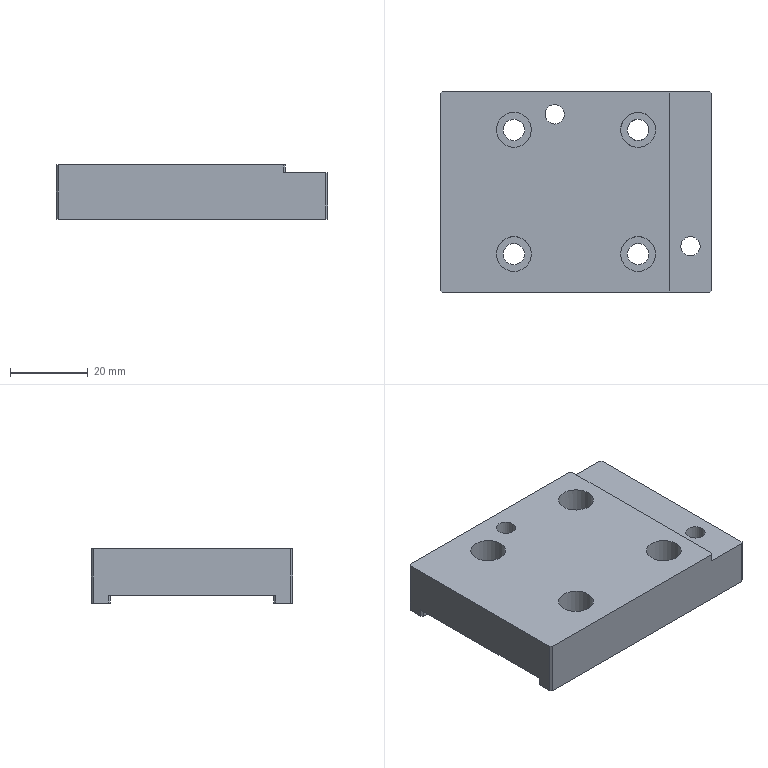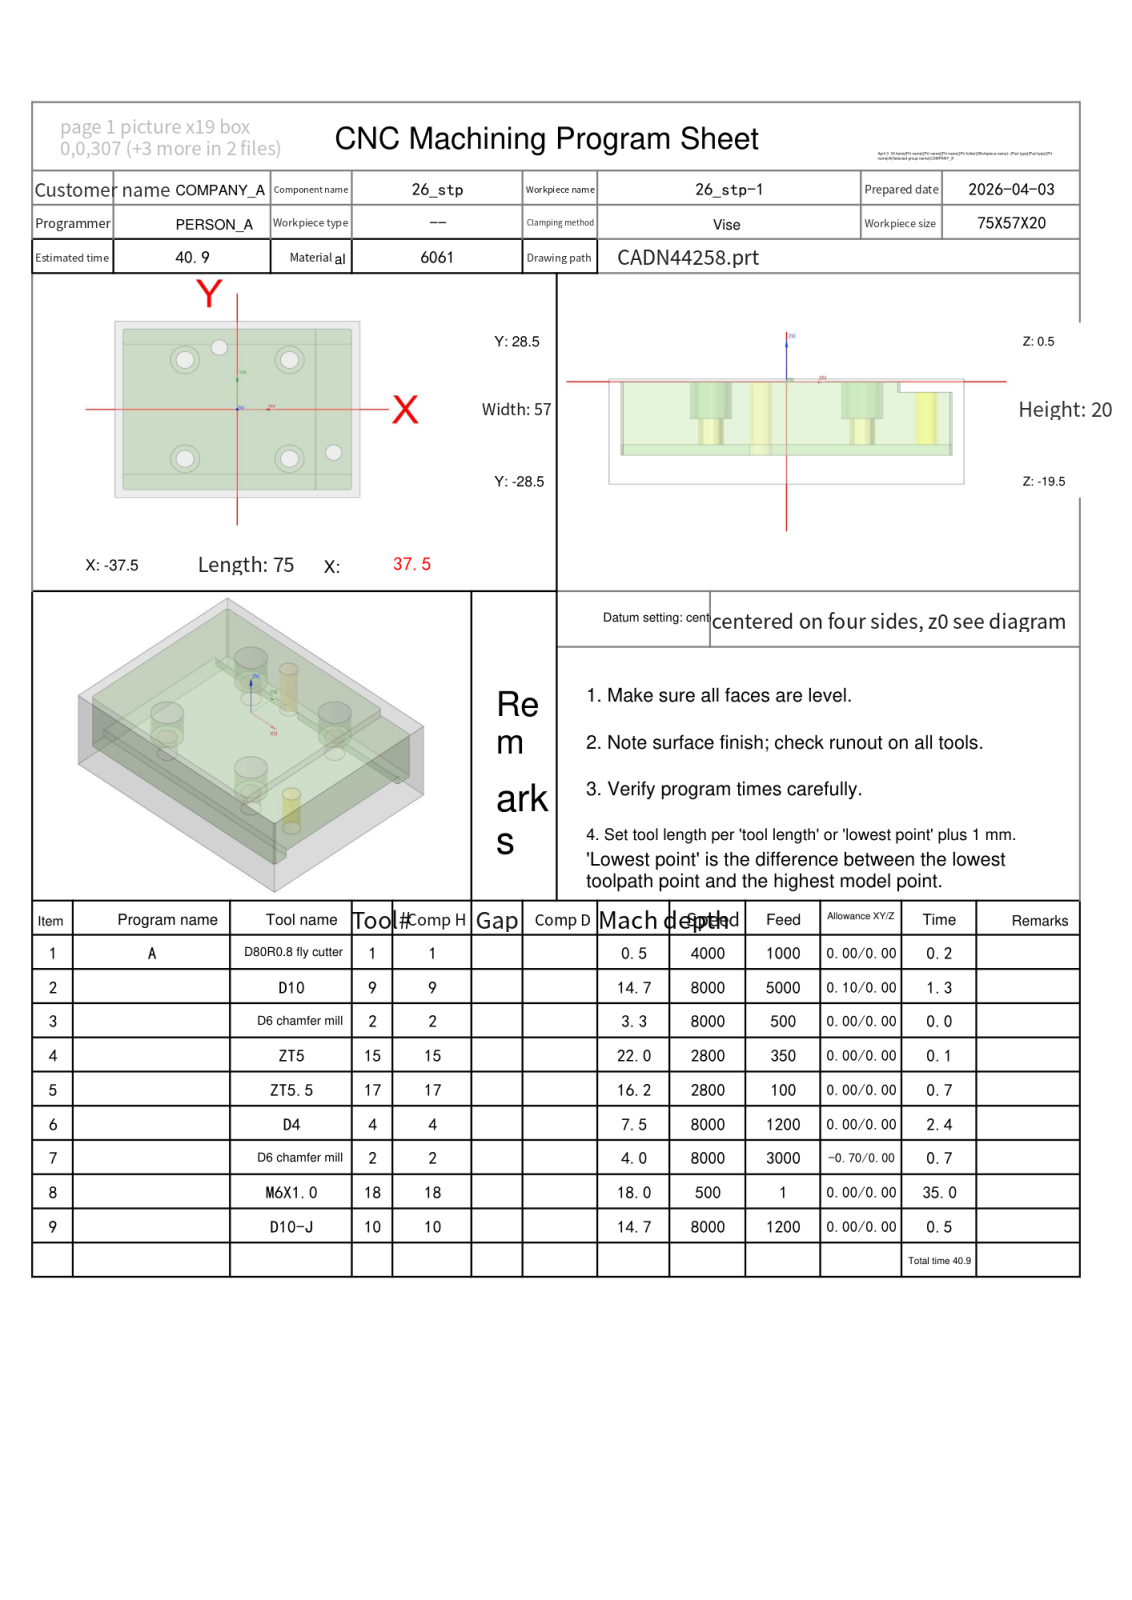NC program | NX | posted by the shop | part box 70 x 52 x 14 mm
Whole program, first 1466 of 2128 lines:
%
O0001
(Machine time: 75.66 MIN)
(===Total Tool:8===)
(T1=D80R0.8 fly cutter D=80.  R=0.8  D-  H01 Z=0.    )
(T9=D10     D=10.  R=0.   D-  H09 Z=-14.2 )
(T2=D6 chamfer mill   D=6.   R=0.   D-  H02 Z=-3.5  )
(T15=ZT5    D=5.   DR_a=118 D-  H15 Z=-21.5 )
(T17=ZT5.5  D=5.5  DR_a=118 D-  H17 Z=-15.65)
(T4=D4      D=4.   R=0.   D4  H04 Z=-7.   )
(T18=M6X1.0 D=5.   DR_a=180 D-  H18 Z=-17.5 )
(T10=D10-J  D=10.  R=0.   D10 H10 Z=-14.2 )
G80 G90 G17 G49 G40
G91 G28 Z0
M01
N1 T01 M06
(D80R0.8 fly cutter  D=80. R=0.8 H=01 ce=0.00 di=0.00)
G00 G90 G54 X-80. Y0.0 M03 S4000
G43 H01 Z20.
M08
Z2.
G01 Z0.0 F1000.
X-75.
X75.
X80.
Z2.
G00 Z20.
G91 G28 Z0.0
M05
M09
G91 G28 Z0.0
M01
N2 T09 M06
(D10  D=10. R=0. H=09 ce=0.10 di=0.00)
G00 G90 G54 X0.0 Y31.1 M03 S8000
G43 H09 Z20.
M08
Z.5
G01 X34.5 Z.403 F5000.
G02 X38.106 Y29.606 Z.392 I0.0 J-5.1
G01 X38.606 Y29.106 Z.39
G02 X40.1 Y25.5 Z.378 I-3.606 J-3.606
G01 Y-25.5 Z.235
G02 X38.606 Y-29.106 Z.224 I-5.1 J0.0
G01 X38.106 Y-29.606 Z.222
G02 X34.5 Y-31.1 Z.21 I-3.606 J3.606
G01 X-34.5 Z.016
G02 X-38.106 Y-29.606 Z.005 I0.0 J5.1
G01 X-38.606 Y-29.106 Z.003
G02 X-40.1 Y-25.5 Z-.008 I3.606 J3.606
G01 Y25.5 Z-.152
G02 X-38.606 Y29.106 Z-.163 I5.1 J0.0
G01 X-38.106 Y29.606 Z-.165
G02 X-34.5 Y31.1 Z-.177 I3.606 J-3.606
G01 X34.5 Z-.371
G02 X38.106 Y29.606 Z-.382 I0.0 J-5.1
G01 X38.606 Y29.106 Z-.384
G02 X40.1 Y25.5 Z-.395 I-3.606 J-3.606
G01 Y-25.5 Z-.539
G02 X38.606 Y-29.106 Z-.55 I-5.1 J0.0
G01 X38.106 Y-29.606 Z-.552
G02 X34.5 Y-31.1 Z-.563 I-3.606 J3.606
G01 X-34.5 Z-.758
G02 X-38.106 Y-29.606 Z-.769 I0.0 J5.1
G01 X-38.606 Y-29.106 Z-.771
G02 X-40.1 Y-25.5 Z-.782 I3.606 J3.606
G01 Y25.5 Z-.926
G02 X-38.606 Y29.106 Z-.937 I5.1 J0.0
G01 X-38.106 Y29.606 Z-.939
G02 X-34.5 Y31.1 Z-.95 I3.606 J-3.606
G01 X34.5 Z-1.144
G02 X38.106 Y29.606 Z-1.156 I0.0 J-5.1
G01 X38.606 Y29.106 Z-1.158
G02 X40.1 Y25.5 Z-1.169 I-3.606 J-3.606
G01 Y-25.5 Z-1.313
G02 X38.606 Y-29.106 Z-1.324 I-5.1 J0.0
G01 X38.106 Y-29.606 Z-1.326
G02 X34.5 Y-31.1 Z-1.337 I-3.606 J3.606
G01 X-34.5 Z-1.531
G02 X-38.106 Y-29.606 Z-1.543 I0.0 J5.1
G01 X-38.606 Y-29.106 Z-1.545
G02 X-40.1 Y-25.5 Z-1.556 I3.606 J3.606
G01 Y25.5 Z-1.699
G02 X-38.606 Y29.106 Z-1.711 I5.1 J0.0
G01 X-38.106 Y29.606 Z-1.713
G02 X-34.5 Y31.1 Z-1.724 I3.606 J-3.606
G01 X34.5 Z-1.918
G02 X38.106 Y29.606 Z-1.929 I0.0 J-5.1
G01 X38.606 Y29.106 Z-1.931
G02 X40.1 Y25.5 Z-1.943 I-3.606 J-3.606
G01 Y-25.5 Z-2.086
G02 X38.606 Y-29.106 Z-2.098 I-5.1 J0.0
G01 X38.106 Y-29.606 Z-2.1
G02 X34.5 Y-31.1 Z-2.111 I-3.606 J3.606
G01 X-34.5 Z-2.305
G02 X-38.106 Y-29.606 Z-2.316 I0.0 J5.1
G01 X-38.606 Y-29.106 Z-2.318
G02 X-40.1 Y-25.5 Z-2.33 I3.606 J3.606
G01 Y25.5 Z-2.473
G02 X-38.606 Y29.106 Z-2.484 I5.1 J0.0
G01 X-38.106 Y29.606 Z-2.486
G02 X-34.5 Y31.1 Z-2.498 I3.606 J-3.606
G01 X34.5 Z-2.692
G02 X38.106 Y29.606 Z-2.703 I0.0 J-5.1
G01 X38.606 Y29.106 Z-2.705
G02 X40.1 Y25.5 Z-2.716 I-3.606 J-3.606
G01 Y-25.5 Z-2.86
G02 X38.606 Y-29.106 Z-2.871 I-5.1 J0.0
G01 X38.106 Y-29.606 Z-2.873
G02 X34.5 Y-31.1 Z-2.884 I-3.606 J3.606
G01 X-34.5 Z-3.079
G02 X-38.106 Y-29.606 Z-3.09 I0.0 J5.1
G01 X-38.606 Y-29.106 Z-3.092
G02 X-40.1 Y-25.5 Z-3.103 I3.606 J3.606
G01 Y25.5 Z-3.247
G02 X-38.606 Y29.106 Z-3.258 I5.1 J0.0
G01 X-38.106 Y29.606 Z-3.26
G02 X-34.5 Y31.1 Z-3.271 I3.606 J-3.606
G01 X34.5 Z-3.466
G02 X38.106 Y29.606 Z-3.477 I0.0 J-5.1
G01 X38.606 Y29.106 Z-3.479
G02 X40.1 Y25.5 Z-3.49 I-3.606 J-3.606
G01 Y-25.5 Z-3.634
G02 X38.606 Y-29.106 Z-3.645 I-5.1 J0.0
G01 X38.106 Y-29.606 Z-3.647
G02 X34.5 Y-31.1 Z-3.658 I-3.606 J3.606
G01 X-34.5 Z-3.852
G02 X-38.106 Y-29.606 Z-3.864 I0.0 J5.1
G01 X-38.606 Y-29.106 Z-3.866
G02 X-40.1 Y-25.5 Z-3.877 I3.606 J3.606
G01 Y25.5 Z-4.02
G02 X-38.606 Y29.106 Z-4.032 I5.1 J0.0
G01 X-38.106 Y29.606 Z-4.034
G02 X-34.5 Y31.1 Z-4.045 I3.606 J-3.606
G01 X34.5 Z-4.239
G02 X38.106 Y29.606 Z-4.25 I0.0 J-5.1
G01 X38.606 Y29.106 Z-4.252
G02 X40.1 Y25.5 Z-4.264 I-3.606 J-3.606
G01 Y-25.5 Z-4.407
G02 X38.606 Y-29.106 Z-4.419 I-5.1 J0.0
G01 X38.106 Y-29.606 Z-4.421
G02 X34.5 Y-31.1 Z-4.432 I-3.606 J3.606
G01 X-34.5 Z-4.626
G02 X-38.106 Y-29.606 Z-4.637 I0.0 J5.1
G01 X-38.606 Y-29.106 Z-4.639
G02 X-40.1 Y-25.5 Z-4.651 I3.606 J3.606
G01 Y25.5 Z-4.794
G02 X-38.606 Y29.106 Z-4.805 I5.1 J0.0
G01 X-38.106 Y29.606 Z-4.807
G02 X-34.5 Y31.1 Z-4.819 I3.606 J-3.606
G01 X34.5 Z-5.013
G02 X38.106 Y29.606 Z-5.024 I0.0 J-5.1
G01 X38.606 Y29.106 Z-5.026
G02 X40.1 Y25.5 Z-5.037 I-3.606 J-3.606
G01 Y-25.5 Z-5.181
G02 X38.606 Y-29.106 Z-5.192 I-5.1 J0.0
G01 X38.106 Y-29.606 Z-5.194
G02 X34.5 Y-31.1 Z-5.206 I-3.606 J3.606
G01 X-34.5 Z-5.4
G02 X-38.106 Y-29.606 Z-5.411 I0.0 J5.1
G01 X-38.606 Y-29.106 Z-5.413
G02 X-40.1 Y-25.5 Z-5.424 I3.606 J3.606
G01 Y25.5 Z-5.568
G02 X-38.606 Y29.106 Z-5.579 I5.1 J0.0
G01 X-38.106 Y29.606 Z-5.581
G02 X-34.5 Y31.1 Z-5.592 I3.606 J-3.606
G01 X34.5 Z-5.787
G02 X38.106 Y29.606 Z-5.798 I0.0 J-5.1
G01 X38.606 Y29.106 Z-5.8
G02 X40.1 Y25.5 Z-5.811 I-3.606 J-3.606
G01 Y-25.5 Z-5.955
G02 X38.606 Y-29.106 Z-5.966 I-5.1 J0.0
G01 X38.106 Y-29.606 Z-5.968
G02 X34.5 Y-31.1 Z-5.979 I-3.606 J3.606
G01 X-34.5 Z-6.173
G02 X-38.106 Y-29.606 Z-6.185 I0.0 J5.1
G01 X-38.606 Y-29.106 Z-6.187
G02 X-40.1 Y-25.5 Z-6.198 I3.606 J3.606
G01 Y25.5 Z-6.342
G02 X-38.606 Y29.106 Z-6.353 I5.1 J0.0
G01 X-38.106 Y29.606 Z-6.355
G02 X-34.5 Y31.1 Z-6.366 I3.606 J-3.606
G01 X34.5 Z-6.56
G02 X38.106 Y29.606 Z-6.572 I0.0 J-5.1
G01 X38.606 Y29.106 Z-6.574
G02 X40.1 Y25.5 Z-6.585 I-3.606 J-3.606
G01 Y-25.5 Z-6.728
G02 X38.606 Y-29.106 Z-6.74 I-5.1 J0.0
G01 X38.106 Y-29.606 Z-6.742
G02 X34.5 Y-31.1 Z-6.753 I-3.606 J3.606
G01 X-34.5 Z-6.947
G02 X-38.106 Y-29.606 Z-6.958 I0.0 J5.1
G01 X-38.606 Y-29.106 Z-6.96
G02 X-40.1 Y-25.5 Z-6.972 I3.606 J3.606
G01 Y25.5 Z-7.115
G02 X-38.606 Y29.106 Z-7.126 I5.1 J0.0
G01 X-38.106 Y29.606 Z-7.128
G02 X-34.5 Y31.1 Z-7.14 I3.606 J-3.606
G01 X34.5 Z-7.334
G02 X38.106 Y29.606 Z-7.345 I0.0 J-5.1
G01 X38.606 Y29.106 Z-7.347
G02 X40.1 Y25.5 Z-7.358 I-3.606 J-3.606
G01 Y-25.5 Z-7.502
G02 X38.606 Y-29.106 Z-7.513 I-5.1 J0.0
G01 X38.106 Y-29.606 Z-7.515
G02 X34.5 Y-31.1 Z-7.527 I-3.606 J3.606
G01 X-34.5 Z-7.721
G02 X-38.106 Y-29.606 Z-7.732 I0.0 J5.1
G01 X-38.606 Y-29.106 Z-7.734
G02 X-40.1 Y-25.5 Z-7.745 I3.606 J3.606
G01 Y25.5 Z-7.889
G02 X-38.606 Y29.106 Z-7.9 I5.1 J0.0
G01 X-38.106 Y29.606 Z-7.902
G02 X-34.5 Y31.1 Z-7.913 I3.606 J-3.606
G01 X34.5 Z-8.108
G02 X38.106 Y29.606 Z-8.119 I0.0 J-5.1
G01 X38.606 Y29.106 Z-8.121
G02 X40.1 Y25.5 Z-8.132 I-3.606 J-3.606
G01 Y-25.5 Z-8.276
G02 X38.606 Y-29.106 Z-8.287 I-5.1 J0.0
G01 X38.106 Y-29.606 Z-8.289
G02 X34.5 Y-31.1 Z-8.3 I-3.606 J3.606
G01 X-34.5 Z-8.494
G02 X-38.106 Y-29.606 Z-8.506 I0.0 J5.1
G01 X-38.606 Y-29.106 Z-8.508
G02 X-40.1 Y-25.5 Z-8.519 I3.606 J3.606
G01 Y25.5 Z-8.663
G02 X-38.606 Y29.106 Z-8.674 I5.1 J0.0
G01 X-38.106 Y29.606 Z-8.676
G02 X-34.5 Y31.1 Z-8.687 I3.606 J-3.606
G01 X34.5 Z-8.881
G02 X38.106 Y29.606 Z-8.893 I0.0 J-5.1
G01 X38.606 Y29.106 Z-8.895
G02 X40.1 Y25.5 Z-8.906 I-3.606 J-3.606
G01 Y-25.5 Z-9.049
G02 X38.606 Y-29.106 Z-9.061 I-5.1 J0.0
G01 X38.106 Y-29.606 Z-9.063
G02 X34.5 Y-31.1 Z-9.074 I-3.606 J3.606
G01 X-34.5 Z-9.268
G02 X-38.106 Y-29.606 Z-9.279 I0.0 J5.1
G01 X-38.606 Y-29.106 Z-9.281
G02 X-40.1 Y-25.5 Z-9.293 I3.606 J3.606
G01 Y25.5 Z-9.436
G02 X-38.606 Y29.106 Z-9.448 I5.1 J0.0
G01 X-38.106 Y29.606 Z-9.45
G02 X-34.5 Y31.1 Z-9.461 I3.606 J-3.606
G01 X34.5 Z-9.655
G02 X38.106 Y29.606 Z-9.666 I0.0 J-5.1
G01 X38.606 Y29.106 Z-9.668
G02 X40.1 Y25.5 Z-9.68 I-3.606 J-3.606
G01 Y-25.5 Z-9.823
G02 X38.606 Y-29.106 Z-9.834 I-5.1 J0.0
G01 X38.106 Y-29.606 Z-9.836
G02 X34.5 Y-31.1 Z-9.848 I-3.606 J3.606
G01 X-34.5 Z-10.042
G02 X-38.106 Y-29.606 Z-10.053 I0.0 J5.1
G01 X-38.606 Y-29.106 Z-10.055
G02 X-40.1 Y-25.5 Z-10.066 I3.606 J3.606
G01 Y25.5 Z-10.21
G02 X-38.606 Y29.106 Z-10.221 I5.1 J0.0
G01 X-38.106 Y29.606 Z-10.223
G02 X-34.5 Y31.1 Z-10.234 I3.606 J-3.606
G01 X34.5 Z-10.429
G02 X38.106 Y29.606 Z-10.44 I0.0 J-5.1
G01 X38.606 Y29.106 Z-10.442
G02 X40.1 Y25.5 Z-10.453 I-3.606 J-3.606
G01 Y-25.5 Z-10.597
G02 X38.606 Y-29.106 Z-10.608 I-5.1 J0.0
G01 X38.106 Y-29.606 Z-10.61
G02 X34.5 Y-31.1 Z-10.621 I-3.606 J3.606
G01 X-34.5 Z-10.816
G02 X-38.106 Y-29.606 Z-10.827 I0.0 J5.1
G01 X-38.606 Y-29.106 Z-10.829
G02 X-40.1 Y-25.5 Z-10.84 I3.606 J3.606
G01 Y25.5 Z-10.984
G02 X-38.606 Y29.106 Z-10.995 I5.1 J0.0
G01 X-38.106 Y29.606 Z-10.997
G02 X-34.5 Y31.1 Z-11.008 I3.606 J-3.606
G01 X34.5 Z-11.202
G02 X38.106 Y29.606 Z-11.214 I0.0 J-5.1
G01 X38.606 Y29.106 Z-11.216
G02 X40.1 Y25.5 Z-11.227 I-3.606 J-3.606
G01 Y-25.5 Z-11.37
G02 X38.606 Y-29.106 Z-11.382 I-5.1 J0.0
G01 X38.106 Y-29.606 Z-11.384
G02 X34.5 Y-31.1 Z-11.395 I-3.606 J3.606
G01 X-34.5 Z-11.589
G02 X-38.106 Y-29.606 Z-11.6 I0.0 J5.1
G01 X-38.606 Y-29.106 Z-11.602
G02 X-40.1 Y-25.5 Z-11.614 I3.606 J3.606
G01 Y25.5 Z-11.757
G02 X-38.606 Y29.106 Z-11.769 I5.1 J0.0
G01 X-38.106 Y29.606 Z-11.771
G02 X-34.5 Y31.1 Z-11.782 I3.606 J-3.606
G01 X34.5 Z-11.976
G02 X38.106 Y29.606 Z-11.987 I0.0 J-5.1
G01 X38.606 Y29.106 Z-11.989
G02 X40.1 Y25.5 Z-12.001 I-3.606 J-3.606
G01 Y-25.5 Z-12.144
G02 X38.606 Y-29.106 Z-12.155 I-5.1 J0.0
G01 X38.106 Y-29.606 Z-12.157
G02 X34.5 Y-31.1 Z-12.169 I-3.606 J3.606
G01 X-34.5 Z-12.363
G02 X-38.106 Y-29.606 Z-12.374 I0.0 J5.1
G01 X-38.606 Y-29.106 Z-12.376
G02 X-40.1 Y-25.5 Z-12.387 I3.606 J3.606
G01 Y25.5 Z-12.531
G02 X-38.606 Y29.106 Z-12.542 I5.1 J0.0
G01 X-38.106 Y29.606 Z-12.544
G02 X-34.5 Y31.1 Z-12.556 I3.606 J-3.606
G01 X34.5 Z-12.75
G02 X38.106 Y29.606 Z-12.761 I0.0 J-5.1
G01 X38.606 Y29.106 Z-12.763
G02 X40.1 Y25.5 Z-12.774 I-3.606 J-3.606
G01 Y-25.5 Z-12.918
G02 X38.606 Y-29.106 Z-12.929 I-5.1 J0.0
G01 X38.106 Y-29.606 Z-12.931
G02 X34.5 Y-31.1 Z-12.942 I-3.606 J3.606
G01 X-34.5 Z-13.137
G02 X-38.106 Y-29.606 Z-13.148 I0.0 J5.1
G01 X-38.606 Y-29.106 Z-13.15
G02 X-40.1 Y-25.5 Z-13.161 I3.606 J3.606
G01 Y25.5 Z-13.305
G02 X-38.606 Y29.106 Z-13.316 I5.1 J0.0
G01 X-38.106 Y29.606 Z-13.318
G02 X-34.5 Y31.1 Z-13.329 I3.606 J-3.606
G01 X34.5 Z-13.523
G02 X38.106 Y29.606 Z-13.535 I0.0 J-5.1
G01 X38.606 Y29.106 Z-13.537
G02 X40.1 Y25.5 Z-13.548 I-3.606 J-3.606
G01 Y-25.5 Z-13.692
G02 X38.606 Y-29.106 Z-13.703 I-5.1 J0.0
G01 X38.106 Y-29.606 Z-13.705
G02 X34.5 Y-31.1 Z-13.716 I-3.606 J3.606
G01 X-34.5 Z-13.91
G02 X-38.106 Y-29.606 Z-13.922 I0.0 J5.1
G01 X-38.606 Y-29.106 Z-13.924
G02 X-40.1 Y-25.5 Z-13.935 I3.606 J3.606
G01 Y25.5 Z-14.078
G02 X-38.606 Y29.106 Z-14.09 I5.1 J0.0
G01 X-38.106 Y29.606 Z-14.092
G02 X-34.5 Y31.1 Z-14.103 I3.606 J-3.606
G01 X0.0 Z-14.2
X34.5
G02 X38.106 Y29.606 I0.0 J-5.1
G01 X38.606 Y29.106
G02 X40.1 Y25.5 I-3.606 J-3.606
G01 Y-25.5
G02 X38.606 Y-29.106 I-5.1 J0.0
G01 X38.106 Y-29.606
G02 X34.5 Y-31.1 I-3.606 J3.606
G01 X-34.5
G02 X-38.106 Y-29.606 I0.0 J5.1
G01 X-38.606 Y-29.106
G02 X-40.1 Y-25.5 I3.606 J3.606
G01 Y25.5
G02 X-38.606 Y29.106 I5.1 J0.0
G01 X-38.106 Y29.606
G02 X-34.5 Y31.1 I3.606 J-3.606
G01 X0.0
X.5
Z-13.2
G00 Z20.
G00 G90 X43. Y0.0 M03 S6000
Z20.
Z.025
G01 Z-.475 F3500.
X36.
Y25.914
X34.914 Y27.
X29.1
Y-27.
X34.914
X36. Y-25.914
Y0.0
Y.5
Z.025
G00 Z.5
X43. Y0.0
Z-.45
G01 Z-.95
X36.
Y25.914
X34.914 Y27.
X29.1
Y-27.
X34.914
X36. Y-25.914
Y0.0
Y.5
Z-.45
G00 Z.025
X43. Y0.0
Z-.925
G01 Z-1.425
X36.
Y25.914
X34.914 Y27.
X29.1
Y-27.
X34.914
X36. Y-25.914
Y0.0
Y.5
Z-.925
G00 Z-.45
X43. Y0.0
Z-1.4
G01 Z-1.9
X36.
Y25.914
X34.914 Y27.
X29.1
Y-27.
X34.914
X36. Y-25.914
Y0.0
Y.5
Z-1.4
G00 Z20.
G91 G28 Z0.0
M05
M09
G91 G28 Z0.0
M01
N3 T02 M06
(D6 chamfer mill  D=6. R=0. H=02 ce=0.00 di=0.10)
G00 G90 G54 X29.5 Y-14. M03 S8000
G43 H02 Z20.
M08
G98 G81 X29.5 Y-14. Z-2.8 R-1. F500.
X16. Y-16. Z-.8 R1.
Y16.
X-5.5 Y20.
X-16. Y16.
Y-16.
G80
G00 Z20.
G91 G28 Z0.0
M05
M09
G91 G28 Z0.0
M01
N4 T15 M06
(ZT5 D=5. DR_a=118 H=15)
G00 G90 G54 X29.5 Y-14. M03 S2800
G43 H15 Z20.
M08
G98 G83 X29.5 Y-14. Z-19.502 R-1. F350. Q3.
G98 G83 X-5.5 Y20. Z-21.502 R1. Q3.
G80
G00 Z20.
G91 G28 Z0.0
M05
M09
G91 G28 Z0.0
M01
N5 T17 M06
(ZT5.5 D=5.5 DR_a=118 H=17)
G00 G90 G54 X16. Y16. M03 S2800
G43 H17 Z20.
M08
G98 G83 X16. Y16. Z-15.652 R1. F100. Q2.
Y-16.
X-16.
Y16.
G80
G00 Z20.
G91 G28 Z0.0
M05
M09
G91 G28 Z0.0
M01
N6 T04 M06
(D4  D=4. R=0. H=04 ce=0.10 di=0.00)
G00 G90 G54 X16. Y16. M03 S8000
G43 H04 Z20.
M08
Z.5
G03 X16.6 Y15.4 I.6 J0.0 F1200.
X17.2 Y16. I0.0 J.6
X17.2 Y16. Z.2 I-1.2 J0.0
X17.2 Y16. Z-.1 I-1.2 J0.0
X17.2 Y16. Z-.4 I-1.2 J0.0
X17.2 Y16. Z-.7 I-1.2 J0.0
X17.2 Y16. Z-1. I-1.2 J0.0
X17.2 Y16. Z-1.3 I-1.2 J0.0
X17.2 Y16. Z-1.6 I-1.2 J0.0
X17.2 Y16. Z-1.9 I-1.2 J0.0
X17.2 Y16. Z-2.2 I-1.2 J0.0
X17.2 Y16. Z-2.5 I-1.2 J0.0
X17.2 Y16. Z-2.8 I-1.2 J0.0
X17.2 Y16. Z-3.1 I-1.2 J0.0
X17.2 Y16. Z-3.4 I-1.2 J0.0
X17.2 Y16. Z-3.7 I-1.2 J0.0
X17.2 Y16. Z-4. I-1.2 J0.0
X17.2 Y16. Z-4.3 I-1.2 J0.0
X17.2 Y16. Z-4.6 I-1.2 J0.0
X17.2 Y16. Z-4.9 I-1.2 J0.0
X17.2 Y16. Z-5.2 I-1.2 J0.0
X17.2 Y16. Z-5.5 I-1.2 J0.0
X17.2 Y16. Z-5.8 I-1.2 J0.0
X17.2 Y16. Z-6.1 I-1.2 J0.0
X17.2 Y16. Z-6.4 I-1.2 J0.0
X17.2 Y16. Z-6.7 I-1.2 J0.0
X17.2 Y16. Z-7. I-1.2 J0.0
X16. Y17.2 I-1.2 J0.0
X14.8 Y16. I0.0 J-1.2
X16. Y14.8 I1.2 J0.0
X17.2 Y16. I0.0 J1.2
X16.6 Y16.6 I-.6 J0.0
X16. Y16. I0.0 J-.6
G00 Z.5
G03 X17.2 Y14.8 I1.2 J0.0
X18.4 Y16. I0.0 J1.2
X18.4 Y16. Z.2 I-2.4 J0.0
X18.4 Y16. Z-.1 I-2.4 J0.0
X18.4 Y16. Z-.4 I-2.4 J0.0
X18.4 Y16. Z-.7 I-2.4 J0.0
X18.4 Y16. Z-1. I-2.4 J0.0
X18.4 Y16. Z-1.3 I-2.4 J0.0
X18.4 Y16. Z-1.6 I-2.4 J0.0
X18.4 Y16. Z-1.9 I-2.4 J0.0
X18.4 Y16. Z-2.2 I-2.4 J0.0
X18.4 Y16. Z-2.5 I-2.4 J0.0
X18.4 Y16. Z-2.8 I-2.4 J0.0
X18.4 Y16. Z-3.1 I-2.4 J0.0
X18.4 Y16. Z-3.4 I-2.4 J0.0
X18.4 Y16. Z-3.7 I-2.4 J0.0
X18.4 Y16. Z-4. I-2.4 J0.0
X18.4 Y16. Z-4.3 I-2.4 J0.0
X18.4 Y16. Z-4.6 I-2.4 J0.0
X18.4 Y16. Z-4.9 I-2.4 J0.0
X18.4 Y16. Z-5.2 I-2.4 J0.0
X18.4 Y16. Z-5.5 I-2.4 J0.0
X18.4 Y16. Z-5.8 I-2.4 J0.0
X18.4 Y16. Z-6.1 I-2.4 J0.0
X18.4 Y16. Z-6.4 I-2.4 J0.0
X18.4 Y16. Z-6.7 I-2.4 J0.0
X18.4 Y16. Z-7. I-2.4 J0.0
X16. Y18.4 I-2.4 J0.0
X13.6 Y16. I0.0 J-2.4
X16. Y13.6 I2.4 J0.0
X18.4 Y16. I0.0 J2.4
X17.2 Y17.2 I-1.2 J0.0
X16. Y16. I0.0 J-1.2
G00 Z20.
Y-16.
Z.5
G03 X16.6 Y-16.6 I.6 J0.0
X17.2 Y-16. I0.0 J.6
X17.2 Y-16. Z.2 I-1.2 J0.0
X17.2 Y-16. Z-.1 I-1.2 J0.0
X17.2 Y-16. Z-.4 I-1.2 J0.0
X17.2 Y-16. Z-.7 I-1.2 J0.0
X17.2 Y-16. Z-1. I-1.2 J0.0
X17.2 Y-16. Z-1.3 I-1.2 J0.0
X17.2 Y-16. Z-1.6 I-1.2 J0.0
X17.2 Y-16. Z-1.9 I-1.2 J0.0
X17.2 Y-16. Z-2.2 I-1.2 J0.0
X17.2 Y-16. Z-2.5 I-1.2 J0.0
X17.2 Y-16. Z-2.8 I-1.2 J0.0
X17.2 Y-16. Z-3.1 I-1.2 J0.0
X17.2 Y-16. Z-3.4 I-1.2 J0.0
X17.2 Y-16. Z-3.7 I-1.2 J0.0
X17.2 Y-16. Z-4. I-1.2 J0.0
X17.2 Y-16. Z-4.3 I-1.2 J0.0
X17.2 Y-16. Z-4.6 I-1.2 J0.0
X17.2 Y-16. Z-4.9 I-1.2 J0.0
X17.2 Y-16. Z-5.2 I-1.2 J0.0
X17.2 Y-16. Z-5.5 I-1.2 J0.0
X17.2 Y-16. Z-5.8 I-1.2 J0.0
X17.2 Y-16. Z-6.1 I-1.2 J0.0
X17.2 Y-16. Z-6.4 I-1.2 J0.0
X17.2 Y-16. Z-6.7 I-1.2 J0.0
X17.2 Y-16. Z-7. I-1.2 J0.0
X16. Y-14.8 I-1.2 J0.0
X14.8 Y-16. I0.0 J-1.2
X16. Y-17.2 I1.2 J0.0
X17.2 Y-16. I0.0 J1.2
X16.6 Y-15.4 I-.6 J0.0
X16. Y-16. I0.0 J-.6
G00 Z.5
G03 X17.2 Y-17.2 I1.2 J0.0
X18.4 Y-16. I0.0 J1.2
X18.4 Y-16. Z.2 I-2.4 J0.0
X18.4 Y-16. Z-.1 I-2.4 J0.0
X18.4 Y-16. Z-.4 I-2.4 J0.0
X18.4 Y-16. Z-.7 I-2.4 J0.0
X18.4 Y-16. Z-1. I-2.4 J0.0
X18.4 Y-16. Z-1.3 I-2.4 J0.0
X18.4 Y-16. Z-1.6 I-2.4 J0.0
X18.4 Y-16. Z-1.9 I-2.4 J0.0
X18.4 Y-16. Z-2.2 I-2.4 J0.0
X18.4 Y-16. Z-2.5 I-2.4 J0.0
X18.4 Y-16. Z-2.8 I-2.4 J0.0
X18.4 Y-16. Z-3.1 I-2.4 J0.0
X18.4 Y-16. Z-3.4 I-2.4 J0.0
X18.4 Y-16. Z-3.7 I-2.4 J0.0
X18.4 Y-16. Z-4. I-2.4 J0.0
X18.4 Y-16. Z-4.3 I-2.4 J0.0
X18.4 Y-16. Z-4.6 I-2.4 J0.0
X18.4 Y-16. Z-4.9 I-2.4 J0.0
X18.4 Y-16. Z-5.2 I-2.4 J0.0
X18.4 Y-16. Z-5.5 I-2.4 J0.0
X18.4 Y-16. Z-5.8 I-2.4 J0.0
X18.4 Y-16. Z-6.1 I-2.4 J0.0
X18.4 Y-16. Z-6.4 I-2.4 J0.0
X18.4 Y-16. Z-6.7 I-2.4 J0.0
X18.4 Y-16. Z-7. I-2.4 J0.0
X16. Y-13.6 I-2.4 J0.0
X13.6 Y-16. I0.0 J-2.4
X16. Y-18.4 I2.4 J0.0
X18.4 Y-16. I0.0 J2.4
X17.2 Y-14.8 I-1.2 J0.0
X16. Y-16. I0.0 J-1.2
G00 Z20.
X-16.
Z.5
G03 X-15.4 Y-16.6 I.6 J0.0
X-14.8 Y-16. I0.0 J.6
X-14.8 Y-16. Z.2 I-1.2 J0.0
X-14.8 Y-16. Z-.1 I-1.2 J0.0
X-14.8 Y-16. Z-.4 I-1.2 J0.0
X-14.8 Y-16. Z-.7 I-1.2 J0.0
X-14.8 Y-16. Z-1. I-1.2 J0.0
X-14.8 Y-16. Z-1.3 I-1.2 J0.0
X-14.8 Y-16. Z-1.6 I-1.2 J0.0
X-14.8 Y-16. Z-1.9 I-1.2 J0.0
X-14.8 Y-16. Z-2.2 I-1.2 J0.0
X-14.8 Y-16. Z-2.5 I-1.2 J0.0
X-14.8 Y-16. Z-2.8 I-1.2 J0.0
X-14.8 Y-16. Z-3.1 I-1.2 J0.0
X-14.8 Y-16. Z-3.4 I-1.2 J0.0
X-14.8 Y-16. Z-3.7 I-1.2 J0.0
X-14.8 Y-16. Z-4. I-1.2 J0.0
X-14.8 Y-16. Z-4.3 I-1.2 J0.0
X-14.8 Y-16. Z-4.6 I-1.2 J0.0
X-14.8 Y-16. Z-4.9 I-1.2 J0.0
X-14.8 Y-16. Z-5.2 I-1.2 J0.0
X-14.8 Y-16. Z-5.5 I-1.2 J0.0
X-14.8 Y-16. Z-5.8 I-1.2 J0.0
X-14.8 Y-16. Z-6.1 I-1.2 J0.0
X-14.8 Y-16. Z-6.4 I-1.2 J0.0
X-14.8 Y-16. Z-6.7 I-1.2 J0.0
X-14.8 Y-16. Z-7. I-1.2 J0.0
X-16. Y-14.8 I-1.2 J0.0
X-17.2 Y-16. I0.0 J-1.2
X-16. Y-17.2 I1.2 J0.0
X-14.8 Y-16. I0.0 J1.2
X-15.4 Y-15.4 I-.6 J0.0
X-16. Y-16. I0.0 J-.6
G00 Z.5
G03 X-14.8 Y-17.2 I1.2 J0.0
X-13.6 Y-16. I0.0 J1.2
X-13.6 Y-16. Z.2 I-2.4 J0.0
X-13.6 Y-16. Z-.1 I-2.4 J0.0
X-13.6 Y-16. Z-.4 I-2.4 J0.0
X-13.6 Y-16. Z-.7 I-2.4 J0.0
X-13.6 Y-16. Z-1. I-2.4 J0.0
X-13.6 Y-16. Z-1.3 I-2.4 J0.0
X-13.6 Y-16. Z-1.6 I-2.4 J0.0
X-13.6 Y-16. Z-1.9 I-2.4 J0.0
X-13.6 Y-16. Z-2.2 I-2.4 J0.0
X-13.6 Y-16. Z-2.5 I-2.4 J0.0
X-13.6 Y-16. Z-2.8 I-2.4 J0.0
X-13.6 Y-16. Z-3.1 I-2.4 J0.0
X-13.6 Y-16. Z-3.4 I-2.4 J0.0
X-13.6 Y-16. Z-3.7 I-2.4 J0.0
X-13.6 Y-16. Z-4. I-2.4 J0.0
X-13.6 Y-16. Z-4.3 I-2.4 J0.0
X-13.6 Y-16. Z-4.6 I-2.4 J0.0
X-13.6 Y-16. Z-4.9 I-2.4 J0.0
X-13.6 Y-16. Z-5.2 I-2.4 J0.0
X-13.6 Y-16. Z-5.5 I-2.4 J0.0
X-13.6 Y-16. Z-5.8 I-2.4 J0.0
X-13.6 Y-16. Z-6.1 I-2.4 J0.0
X-13.6 Y-16. Z-6.4 I-2.4 J0.0
X-13.6 Y-16. Z-6.7 I-2.4 J0.0
X-13.6 Y-16. Z-7. I-2.4 J0.0
X-16. Y-13.6 I-2.4 J0.0
X-18.4 Y-16. I0.0 J-2.4
X-16. Y-18.4 I2.4 J0.0
X-13.6 Y-16. I0.0 J2.4
X-14.8 Y-14.8 I-1.2 J0.0
X-16. Y-16. I0.0 J-1.2
G00 Z20.
Y16.
Z.5
G03 X-15.4 Y15.4 I.6 J0.0
X-14.8 Y16. I0.0 J.6
X-14.8 Y16. Z.2 I-1.2 J0.0
X-14.8 Y16. Z-.1 I-1.2 J0.0
X-14.8 Y16. Z-.4 I-1.2 J0.0
X-14.8 Y16. Z-.7 I-1.2 J0.0
X-14.8 Y16. Z-1. I-1.2 J0.0
X-14.8 Y16. Z-1.3 I-1.2 J0.0
X-14.8 Y16. Z-1.6 I-1.2 J0.0
X-14.8 Y16. Z-1.9 I-1.2 J0.0
X-14.8 Y16. Z-2.2 I-1.2 J0.0
X-14.8 Y16. Z-2.5 I-1.2 J0.0
X-14.8 Y16. Z-2.8 I-1.2 J0.0
X-14.8 Y16. Z-3.1 I-1.2 J0.0
X-14.8 Y16. Z-3.4 I-1.2 J0.0
X-14.8 Y16. Z-3.7 I-1.2 J0.0
X-14.8 Y16. Z-4. I-1.2 J0.0
X-14.8 Y16. Z-4.3 I-1.2 J0.0
X-14.8 Y16. Z-4.6 I-1.2 J0.0
X-14.8 Y16. Z-4.9 I-1.2 J0.0
X-14.8 Y16. Z-5.2 I-1.2 J0.0
X-14.8 Y16. Z-5.5 I-1.2 J0.0
X-14.8 Y16. Z-5.8 I-1.2 J0.0
X-14.8 Y16. Z-6.1 I-1.2 J0.0
X-14.8 Y16. Z-6.4 I-1.2 J0.0
X-14.8 Y16. Z-6.7 I-1.2 J0.0
X-14.8 Y16. Z-7. I-1.2 J0.0
X-16. Y17.2 I-1.2 J0.0
X-17.2 Y16. I0.0 J-1.2
X-16. Y14.8 I1.2 J0.0
X-14.8 Y16. I0.0 J1.2
X-15.4 Y16.6 I-.6 J0.0
X-16. Y16. I0.0 J-.6
G00 Z.5
G03 X-14.8 Y14.8 I1.2 J0.0
X-13.6 Y16. I0.0 J1.2
X-13.6 Y16. Z.2 I-2.4 J0.0
X-13.6 Y16. Z-.1 I-2.4 J0.0
X-13.6 Y16. Z-.4 I-2.4 J0.0
X-13.6 Y16. Z-.7 I-2.4 J0.0
X-13.6 Y16. Z-1. I-2.4 J0.0
X-13.6 Y16. Z-1.3 I-2.4 J0.0
X-13.6 Y16. Z-1.6 I-2.4 J0.0
X-13.6 Y16. Z-1.9 I-2.4 J0.0
X-13.6 Y16. Z-2.2 I-2.4 J0.0
X-13.6 Y16. Z-2.5 I-2.4 J0.0
X-13.6 Y16. Z-2.8 I-2.4 J0.0
X-13.6 Y16. Z-3.1 I-2.4 J0.0
X-13.6 Y16. Z-3.4 I-2.4 J0.0
X-13.6 Y16. Z-3.7 I-2.4 J0.0
X-13.6 Y16. Z-4. I-2.4 J0.0
X-13.6 Y16. Z-4.3 I-2.4 J0.0
X-13.6 Y16. Z-4.6 I-2.4 J0.0
X-13.6 Y16. Z-4.9 I-2.4 J0.0
X-13.6 Y16. Z-5.2 I-2.4 J0.0
X-13.6 Y16. Z-5.5 I-2.4 J0.0
X-13.6 Y16. Z-5.8 I-2.4 J0.0
X-13.6 Y16. Z-6.1 I-2.4 J0.0
X-13.6 Y16. Z-6.4 I-2.4 J0.0
X-13.6 Y16. Z-6.7 I-2.4 J0.0
X-13.6 Y16. Z-7. I-2.4 J0.0
X-16. Y18.4 I-2.4 J0.0
X-18.4 Y16. I0.0 J-2.4
X-16. Y13.6 I2.4 J0.0
X-13.6 Y16. I0.0 J2.4
X-14.8 Y17.2 I-1.2 J0.0
X-16. Y16. I0.0 J-1.2
G00 Z20.
G00 G90 X16. Y16. M03 S8000
Z20.
Z.5
G41 D04
G01 X16.032 Y15.803 F500.
G03 X17.258 Y14.758 I1.226 J.197
X18.5 Y16. I0.0 J1.242
X18.5 Y16. Z-4.5 I-2.5 J0.0
X13.5 Y16. Z-7. I-2.5 J0.0
X16. Y13.5 I2.5 J0.0
X18.5 Y16. I0.0 J2.5
X16. Y18.5 I-2.5 J0.0
X13.5 Y16. I0.0 J-2.5
X14.742 Y14.758 I1.242 J0.0
X15.968 Y15.803 I0.0 J1.242
G01 G40 X16. Y16.
G00 Z20.
Y-16.
Z.5
G41 D04
G01 X16.032 Y-16.197
G03 X17.258 Y-17.242 I1.226 J.197
X18.5 Y-16. I0.0 J1.242
X18.5 Y-16. Z-4.5 I-2.5 J0.0
X13.5 Y-16. Z-7. I-2.5 J0.0
X16. Y-18.5 I2.5 J0.0
X18.5 Y-16. I0.0 J2.5
X16. Y-13.5 I-2.5 J0.0
X13.5 Y-16. I0.0 J-2.5
X14.742 Y-17.242 I1.242 J0.0
X15.968 Y-16.197 I0.0 J1.242
G01 G40 X16. Y-16.
G00 Z20.
X-16.
Z.5
G41 D04
G01 X-15.968 Y-16.197
G03 X-14.742 Y-17.242 I1.226 J.197
X-13.5 Y-16. I0.0 J1.242
X-13.5 Y-16. Z-4.5 I-2.5 J0.0
X-18.5 Y-16. Z-7. I-2.5 J0.0
X-16. Y-18.5 I2.5 J0.0
X-13.5 Y-16. I0.0 J2.5
X-16. Y-13.5 I-2.5 J0.0
X-18.5 Y-16. I0.0 J-2.5
X-17.258 Y-17.242 I1.242 J0.0
X-16.032 Y-16.197 I0.0 J1.242
G01 G40 X-16. Y-16.
G00 Z20.
Y16.
Z.5
G41 D04
G01 X-15.968 Y15.803
G03 X-14.742 Y14.758 I1.226 J.197
X-13.5 Y16. I0.0 J1.242
X-13.5 Y16. Z-4.5 I-2.5 J0.0
X-18.5 Y16. Z-7. I-2.5 J0.0
X-16. Y13.5 I2.5 J0.0
X-13.5 Y16. I0.0 J2.5
X-16. Y18.5 I-2.5 J0.0
X-18.5 Y16. I0.0 J-2.5
X-17.258 Y14.758 I1.242 J0.0
X-16.032 Y15.803 I0.0 J1.242
G01 G40 X-16. Y16.
G00 Z20.
G91 G28 Z0.0
M05
M09
G91 G28 Z0.0
M01
N7 T02 M06
(D6 chamfer mill  D=6. R=0. H=02 ce=0.00 di=0.00)
G00 G90 G54 X-5.75 Y28.128 M03 S8000
G43 H02 Z20.
M08
Z2.099
G01 Z-1.5 F3000.
G03 X-5.83 Y27.828 I.52 J-.3
X-5.53 Y27.308 I.6 J0.0
G01 X-5.5 Y27.3
X23.5
X23.754 Y27.275
X23.997 Y27.201
X24.222 Y27.081
X24.419 Y26.919
X24.919 Y26.419
X25.081 Y26.222
X25.201 Y25.997
X25.275 Y25.754
X25.3 Y25.5
Y-25.5
X25.275 Y-25.754
X25.201 Y-25.997
X25.081 Y-26.222
X24.919 Y-26.419
X24.419 Y-26.919
X24.222 Y-27.081
X23.997 Y-27.201
X23.754 Y-27.275
X23.5 Y-27.3
X-34.5
X-34.754 Y-27.275
X-34.997 Y-27.201
X-35.222 Y-27.081
X-35.419 Y-26.919
X-35.919 Y-26.419
X-36.081 Y-26.222
X-36.201 Y-25.997
X-36.275 Y-25.754
X-36.3 Y-25.5
Y25.5
X-36.275 Y25.754
X-36.201 Y25.997
X-36.081 Y26.222
X-35.919 Y26.419
X-35.419 Y26.919
X-35.222 Y27.081
X-34.997 Y27.201
X-34.754 Y27.275
X-34.5 Y27.3
X-5.5
X-5.47 Y27.308
G03 X-5.17 Y27.828 I-.3 J.52
X-5.25 Y28.128 I-.6 J0.0
G01 Z2.099
G00 Z20.
X26.774
Z1.755
G01 Z-3.5
G03 X26.693 Y27.828 I.52 J-.3
X26.993 Y27.308 I.6 J0.0
G01 X27.023 Y27.3
X34.5
X34.754 Y27.275
X34.997 Y27.201
X35.222 Y27.081
X35.419 Y26.919
X35.919 Y26.419
X36.081 Y26.222
X36.201 Y25.997
X36.275 Y25.754
X36.3 Y25.5
Y-25.5
X36.275 Y-25.754
X36.201 Y-25.997
X36.081 Y-26.222
X35.919 Y-26.419
X35.419 Y-26.919
X35.222 Y-27.081
X34.997 Y-27.201
X34.754 Y-27.275
X34.5 Y-27.3
X27.023
X26.993 Y-27.308
G03 X26.693 Y-27.828 I.3 J-.52
X26.774 Y-28.128 I.6 J0.0
G01 Z1.755
G00 Z20.
G00 G90 X29.909 Y-15.021 M03 S8000
Z20.
Z-2.6
G01 Z-3.1 F500.
X30.1 Y-15.5
G03 X31.6 Y-14. I0.0 J1.5
X29.5 Y-11.9 I-2.1 J0.0
X27.4 Y-14. I0.0 J-2.1
X29.5 Y-16.1 I2.1 J0.0
X31.6 Y-14. I0.0 J2.1
X30.1 Y-12.5 I-1.5 J0.0
G01 X29.909 Y-12.979
Z-2.6
G00 Z20.
X-5.3 Y20.008
Z.5
G01 Y20.045 Z.499
X-5.361 Y20.151 Z.494
X-5.439 Y20.196 Z.491
X-5.55 Y20.199 Z.487
X-5.647 Y20.143 Z.484
X-5.7 Y20.045 Z.48
Y19.955 Z.476
X-5.647 Y19.857 Z.473
X-5.55 Y19.801 Z.469
X-5.439 Y19.804 Z.465
X-5.361 Y19.849 Z.462
X-5.3 Y19.955 Z.457
Y20.045 Z.454
X-5.361 Y20.151 Z.45
X-5.439 Y20.196 Z.447
X-5.55 Y20.199 Z.443
X-5.647 Y20.143 Z.439
X-5.7 Y20.045 Z.435
Y19.955 Z.432
X-5.647 Y19.857 Z.428
X-5.55 Y19.801 Z.424
X-5.439 Y19.804 Z.42
X-5.361 Y19.849 Z.417
X-5.3 Y19.955 Z.413
Y20.045 Z.41
X-5.361 Y20.151 Z.406
X-5.439 Y20.196 Z.402
X-5.55 Y20.199 Z.399
X-5.647 Y20.143 Z.395
X-5.7 Y20.045 Z.391
Y19.955 Z.388
X-5.647 Y19.857 Z.384
X-5.55 Y19.801 Z.38
X-5.439 Y19.804 Z.376
X-5.361 Y19.849 Z.373
X-5.3 Y19.955 Z.369
Y20.045 Z.365
X-5.361 Y20.151 Z.361
X-5.439 Y20.196 Z.358
X-5.55 Y20.199 Z.354
X-5.647 Y20.143 Z.35
X-5.7 Y20.045 Z.346
Y19.955 Z.343
X-5.647 Y19.857 Z.339
X-5.55 Y19.801 Z.335
X-5.439 Y19.804 Z.331
X-5.361 Y19.849 Z.328
X-5.3 Y19.955 Z.324
Y20.045 Z.321
X-5.361 Y20.151 Z.317
X-5.439 Y20.196 Z.314
X-5.55 Y20.199 Z.31
X-5.647 Y20.143 Z.306
X-5.7 Y20.045 Z.302
Y19.955 Z.299
X-5.647 Y19.857 Z.295
X-5.55 Y19.801 Z.291
X-5.439 Y19.804 Z.287
X-5.361 Y19.849 Z.284
X-5.3 Y19.955 Z.28
Y20.045 Z.276
X-5.361 Y20.151 Z.272
X-5.439 Y20.196 Z.269
X-5.55 Y20.199 Z.265
X-5.647 Y20.143 Z.261
X-5.7 Y20.045 Z.257
Y19.955 Z.254
X-5.647 Y19.857 Z.25
X-5.55 Y19.801 Z.246
X-5.439 Y19.804 Z.243
X-5.361 Y19.849 Z.239
X-5.3 Y19.955 Z.235
Y20.045 Z.232
X-5.361 Y20.151 Z.228
X-5.439 Y20.196 Z.225
X-5.55 Y20.199 Z.221
X-5.647 Y20.143 Z.217
X-5.7 Y20.045 Z.213
Y19.955 Z.21
X-5.647 Y19.857 Z.206
X-5.55 Y19.801 Z.202
X-5.439 Y19.804 Z.198
X-5.361 Y19.849 Z.195
X-5.3 Y19.955 Z.191
Y20.045 Z.188
X-5.361 Y20.151 Z.183
X-5.439 Y20.196 Z.18
X-5.55 Y20.199 Z.176
X-5.647 Y20.143 Z.172
X-5.7 Y20.045 Z.168
Y19.955 Z.165
X-5.647 Y19.857 Z.161
X-5.55 Y19.801 Z.158
X-5.439 Y19.804 Z.154
X-5.361 Y19.849 Z.151
X-5.3 Y19.955 Z.146
Y20.045 Z.143
X-5.361 Y20.151 Z.139
X-5.439 Y20.196 Z.136
X-5.55 Y20.199 Z.132
X-5.647 Y20.143 Z.128
X-5.7 Y20.045 Z.124
Y19.955 Z.121
X-5.647 Y19.857 Z.117
X-5.55 Y19.801 Z.113
X-5.439 Y19.804 Z.109
X-5.361 Y19.849 Z.106
X-5.3 Y19.955 Z.102
Y20.045 Z.099
X-5.361 Y20.151 Z.094
X-5.439 Y20.196 Z.091
X-5.55 Y20.199 Z.087
X-5.647 Y20.143 Z.083
X-5.7 Y20.045 Z.08
Y19.955 Z.076
X-5.647 Y19.857 Z.073
X-5.55 Y19.801 Z.069
X-5.439 Y19.804 Z.065
X-5.361 Y19.849 Z.062
X-5.3 Y19.955 Z.057
Y20.045 Z.054
X-5.361 Y20.151 Z.05
X-5.439 Y20.196 Z.047
X-5.55 Y20.199 Z.043
X-5.647 Y20.143 Z.039
X-5.7 Y20.045 Z.035
Y19.955 Z.032
X-5.647 Y19.857 Z.028
X-5.55 Y19.801 Z.024
X-5.439 Y19.804 Z.02
X-5.361 Y19.849 Z.017
X-5.3 Y19.955 Z.013
Y20.045 Z.01
X-5.361 Y20.151 Z.006
X-5.439 Y20.196 Z.002
X-5.55 Y20.199 Z-.002
X-5.647 Y20.143 Z-.005
X-5.7 Y20.045 Z-.009
Y19.955 Z-.012
X-5.647 Y19.857 Z-.016
X-5.55 Y19.801 Z-.02
X-5.439 Y19.804 Z-.024
X-5.361 Y19.849 Z-.027
X-5.3 Y19.955 Z-.032
Y20.045 Z-.035
X-5.361 Y20.151 Z-.039
X-5.439 Y20.196 Z-.042
X-5.55 Y20.199 Z-.046
X-5.647 Y20.143 Z-.05
X-5.7 Y20.045 Z-.054
Y19.955 Z-.057
X-5.647 Y19.857 Z-.061
X-5.55 Y19.801 Z-.065
X-5.439 Y19.804 Z-.069
X-5.361 Y19.849 Z-.072
X-5.3 Y19.955 Z-.076
Y20.045 Z-.079
X-5.361 Y20.151 Z-.083
X-5.439 Y20.196 Z-.087
X-5.55 Y20.199 Z-.09
X-5.647 Y20.143 Z-.094
X-5.7 Y20.045 Z-.098
Y19.955 Z-.101
X-5.647 Y19.857 Z-.105
X-5.55 Y19.801 Z-.109
X-5.439 Y19.804 Z-.113
X-5.361 Y19.849 Z-.116
X-5.3 Y19.955 Z-.12
Y20.045 Z-.124
X-5.361 Y20.151 Z-.128
X-5.439 Y20.196 Z-.131
X-5.55 Y20.199 Z-.135
X-5.647 Y20.143 Z-.139
X-5.7 Y20.045 Z-.143
Y19.955 Z-.146
X-5.647 Y19.857 Z-.15
X-5.55 Y19.801 Z-.154
X-5.439 Y19.804 Z-.157
X-5.361 Y19.849 Z-.161
X-5.3 Y19.955 Z-.165
Y20.045 Z-.168
X-5.361 Y20.151 Z-.172
X-5.439 Y20.196 Z-.175
X-5.55 Y20.199 Z-.179
X-5.647 Y20.143 Z-.183
X-5.7 Y20.045 Z-.187
Y19.955 Z-.19
X-5.647 Y19.857 Z-.194
X-5.55 Y19.801 Z-.198
X-5.439 Y19.804 Z-.202
X-5.361 Y19.849 Z-.205
X-5.3 Y19.955 Z-.209
Y20.045 Z-.212
X-5.361 Y20.151 Z-.217
X-5.439 Y20.196 Z-.22
X-5.55 Y20.199 Z-.224
X-5.647 Y20.143 Z-.228
X-5.7 Y20.045 Z-.232
Y19.955 Z-.235
X-5.647 Y19.857 Z-.239
X-5.55 Y19.801 Z-.242
X-5.439 Y19.804 Z-.246
X-5.361 Y19.849 Z-.249
X-5.3 Y19.955 Z-.254
Y20.045 Z-.257
X-5.361 Y20.151 Z-.261
X-5.439 Y20.196 Z-.264
X-5.55 Y20.199 Z-.268
X-5.647 Y20.143 Z-.272
X-5.7 Y20.045 Z-.276
Y19.955 Z-.279
X-5.647 Y19.857 Z-.283
X-5.55 Y19.801 Z-.287
X-5.439 Y19.804 Z-.291
X-5.361 Y19.849 Z-.294
X-5.3 Y19.955 Z-.298
Y20.045 Z-.301
X-5.361 Y20.151 Z-.306
X-5.439 Y20.196 Z-.309
X-5.55 Y20.199 Z-.313
X-5.647 Y20.143 Z-.317
X-5.7 Y20.045 Z-.32
Y19.955 Z-.324
X-5.647 Y19.857 Z-.327
X-5.55 Y19.801 Z-.331
X-5.439 Y19.804 Z-.335
X-5.361 Y19.849 Z-.338
X-5.3 Y19.955 Z-.343
Y20.045 Z-.346
X-5.361 Y20.151 Z-.35
X-5.439 Y20.196 Z-.353
X-5.55 Y20.199 Z-.357
X-5.647 Y20.143 Z-.361
X-5.7 Y20.045 Z-.365
Y19.955 Z-.368
X-5.647 Y19.857 Z-.372
X-5.55 Y19.801 Z-.376
X-5.439 Y19.804 Z-.38
X-5.361 Y19.849 Z-.383
X-5.3 Y19.955 Z-.387
Y20.045 Z-.39
X-5.361 Y20.151 Z-.395
X-5.439 Y20.196 Z-.398
X-5.55 Y20.199 Z-.402
X-5.647 Y20.143 Z-.405
X-5.7 Y20.045 Z-.409
Y19.955 Z-.412
X-5.647 Y19.857 Z-.416
X-5.55 Y19.801 Z-.42
X-5.439 Y19.804 Z-.424
X-5.361 Y19.849 Z-.427
X-5.3 Y19.955 Z-.432
Y20.045 Z-.435
X-5.361 Y20.151 Z-.439
X-5.439 Y20.196 Z-.442
X-5.55 Y20.199 Z-.446
X-5.647 Y20.143 Z-.45
X-5.7 Y20.045 Z-.454
Y19.955 Z-.457
X-5.647 Y19.857 Z-.461
X-5.55 Y19.801 Z-.465
X-5.439 Y19.804 Z-.469
X-5.361 Y19.849 Z-.472
X-5.3 Y19.955 Z-.476
Y20.045 Z-.479
X-5.361 Y20.151 Z-.483
X-5.439 Y20.196 Z-.487
X-5.55 Y20.199 Z-.49
X-5.647 Y20.143 Z-.494
X-5.7 Y20.045 Z-.498
Y19.955 Z-.501
X-5.647 Y19.857 Z-.505
X-5.55 Y19.801 Z-.509
X-5.439 Y19.804 Z-.513
X-5.361 Y19.849 Z-.516
X-5.3 Y19.955 Z-.52
Y20.045 Z-.524
X-5.361 Y20.151 Z-.528
X-5.439 Y20.196 Z-.531
X-5.55 Y20.199 Z-.535
X-5.647 Y20.143 Z-.539
X-5.7 Y20.045 Z-.543
Y19.955 Z-.546
X-5.647 Y19.857 Z-.55
X-5.55 Y19.801 Z-.554
X-5.439 Y19.804 Z-.557
X-5.361 Y19.849 Z-.561
X-5.3 Y19.955 Z-.565
Y20.045 Z-.568
X-5.361 Y20.151 Z-.572
X-5.439 Y20.196 Z-.575
X-5.55 Y20.199 Z-.579
X-5.647 Y20.143 Z-.583
X-5.7 Y20.045 Z-.587
Y19.955 Z-.59
X-5.647 Y19.857 Z-.594
X-5.55 Y19.801 Z-.598
X-5.439 Y19.804 Z-.602
X-5.361 Y19.849 Z-.605
X-5.3 Y19.955 Z-.609
Y20.045 Z-.612
X-5.361 Y20.151 Z-.617
X-5.439 Y20.196 Z-.62
X-5.55 Y20.199 Z-.624
X-5.647 Y20.143 Z-.628
X-5.7 Y20.045 Z-.632
Y19.955 Z-.635
X-5.647 Y19.857 Z-.639
X-5.55 Y19.801 Z-.642
X-5.439 Y19.804 Z-.646
X-5.361 Y19.849 Z-.65
X-5.3 Y19.955 Z-.654
Y20.045 Z-.657
X-5.361 Y20.151 Z-.661
X-5.439 Y20.196 Z-.664
X-5.55 Y20.199 Z-.668
X-5.647 Y20.143 Z-.672
X-5.7 Y20.045 Z-.676
Y19.955 Z-.679
X-5.647 Y19.857 Z-.683
X-5.55 Y19.801 Z-.687
X-5.439 Y19.804 Z-.691
X-5.361 Y19.849 Z-.694
X-5.3 Y19.955 Z-.698
Y20.045 Z-.701
X-5.361 Y20.151 Z-.706
X-5.439 Y20.196 Z-.709
X-5.55 Y20.199 Z-.713
X-5.647 Y20.143 Z-.717
X-5.7 Y20.045 Z-.72
Y19.955 Z-.724
X-5.647 Y19.857 Z-.727
X-5.55 Y19.801 Z-.731
X-5.439 Y19.804 Z-.735
X-5.361 Y19.849 Z-.738
X-5.3 Y19.955 Z-.743
Y20.045 Z-.746
X-5.361 Y20.151 Z-.75
X-5.439 Y20.196 Z-.753
X-5.55 Y20.199 Z-.757
X-5.647 Y20.143 Z-.761
X-5.7 Y20.045 Z-.765
Y19.955 Z-.768
X-5.647 Y19.857 Z-.772
X-5.55 Y19.801 Z-.776
X-5.439 Y19.804 Z-.78
X-5.361 Y19.849 Z-.783
X-5.3 Y19.955 Z-.787
Y20.045 Z-.79
X-5.361 Y20.151 Z-.795
X-5.439 Y20.196 Z-.798
X-5.55 Y20.199 Z-.802
X-5.647 Y20.143 Z-.805
X-5.7 Y20.045 Z-.809
Y19.955 Z-.812
X-5.647 Y19.857 Z-.816
X-5.55 Y19.801 Z-.82
X-5.439 Y19.804 Z-.824
X-5.361 Y19.849 Z-.827
X-5.3 Y19.955 Z-.832
Y20.045 Z-.835
X-5.361 Y20.151 Z-.839
X-5.439 Y20.196 Z-.842
X-5.55 Y20.199 Z-.846
X-5.647 Y20.143 Z-.85
X-5.7 Y20.045 Z-.854
Y19.955 Z-.857
X-5.647 Y19.857 Z-.861
X-5.55 Y19.801 Z-.865
X-5.439 Y19.804 Z-.869
X-5.361 Y19.849 Z-.872
X-5.3 Y19.955 Z-.876
Y20.045 Z-.879
X-5.361 Y20.151 Z-.883
X-5.439 Y20.196 Z-.887
X-5.55 Y20.199 Z-.89
X-5.647 Y20.143 Z-.894
X-5.7 Y20.045 Z-.898
Y19.955 Z-.901
X-5.647 Y19.857 Z-.905
X-5.55 Y19.801 Z-.909
X-5.439 Y19.804 Z-.913
X-5.361 Y19.849 Z-.916
X-5.3 Y19.955 Z-.92
Y20.045 Z-.924
X-5.361 Y20.151 Z-.928
X-5.439 Y20.196 Z-.931
X-5.55 Y20.199 Z-.935
X-5.647 Y20.143 Z-.939
X-5.7 Y20.045 Z-.943
Y19.955 Z-.946
X-5.647 Y19.857 Z-.95
X-5.55 Y19.801 Z-.954
X-5.439 Y19.804 Z-.958
X-5.361 Y19.849 Z-.961
X-5.3 Y19.955 Z-.965
Y20.045 Z-.968
X-5.361 Y20.151 Z-.972
X-5.439 Y20.196 Z-.975
X-5.55 Y20.199 Z-.979
X-5.647 Y20.143 Z-.983
X-5.7 Y20.045 Z-.987
Y19.955 Z-.99
X-5.647 Y19.857 Z-.994
X-5.55 Y19.801 Z-.998
X-5.439 Y19.804 Z-1.002
X-5.361 Y19.849 Z-1.005
X-5.3 Y19.955 Z-1.009
Y20.045 Z-1.013
X-5.361 Y20.151 Z-1.017
X-5.439 Y20.196 Z-1.02
X-5.55 Y20.199 Z-1.024
X-5.647 Y20.143 Z-1.028
X-5.7 Y20.045 Z-1.032
Y19.955 Z-1.035
X-5.647 Y19.857 Z-1.039
X-5.55 Y19.801 Z-1.043
X-5.439 Y19.804 Z-1.046
X-5.361 Y19.849 Z-1.05
X-5.3 Y19.955 Z-1.054
Y20.045 Z-1.057
X-5.361 Y20.151 Z-1.061
X-5.439 Y20.196 Z-1.064
X-5.55 Y20.199 Z-1.068
X-5.647 Y20.143 Z-1.072
X-5.7 Y20.045 Z-1.076
Y19.955 Z-1.079
X-5.647 Y19.857 Z-1.083
X-5.55 Y19.801 Z-1.087
X-5.439 Y19.804 Z-1.091
X-5.361 Y19.849 Z-1.094
X-5.3 Y19.955 Z-1.098
Y20.045 Z-1.101
X-5.361 Y20.151 Z-1.106
X-5.439 Y20.196 Z-1.109
X-5.55 Y20.199 Z-1.113
X-5.647 Y20.143 Z-1.117
X-5.7 Y20.045 Z-1.12
Y19.955 Z-1.124
X-5.647 Y19.857 Z-1.128
X-5.55 Y19.801 Z-1.131
X-5.439 Y19.804 Z-1.135
X-5.361 Y19.849 Z-1.138
X-5.3 Y19.955 Z-1.143
Y20.045 Z-1.146
X-5.361 Y20.151 Z-1.15
X-5.439 Y20.196 Z-1.153
X-5.55 Y20.199 Z-1.157
X-5.647 Y20.143 Z-1.161
X-5.7 Y20.045 Z-1.165
Y19.955 Z-1.168
X-5.647 Y19.857 Z-1.172
X-5.55 Y19.801 Z-1.176
X-5.439 Y19.804 Z-1.18
X-5.361 Y19.849 Z-1.183
X-5.3 Y19.955 Z-1.187
Y20.045 Z-1.19
X-5.361 Y20.151 Z-1.195
X-5.439 Y20.196 Z-1.198
X-5.55 Y20.199 Z-1.202
X-5.647 Y20.143 Z-1.205
X-5.7 Y20.045 Z-1.209
Y19.955 Z-1.213
X-5.647 Y19.857 Z-1.216
X-5.55 Y19.801 Z-1.22
X-5.439 Y19.804 Z-1.224
X-5.361 Y19.849 Z-1.227
X-5.3 Y19.955 Z-1.232
Y20.045 Z-1.235
X-5.361 Y20.151 Z-1.239
X-5.439 Y20.196 Z-1.242
X-5.55 Y20.199 Z-1.246
X-5.647 Y20.143 Z-1.25
X-5.7 Y20.045 Z-1.254
Y19.955 Z-1.257
X-5.647 Y19.857 Z-1.261
X-5.55 Y19.801 Z-1.265
X-5.439 Y19.804 Z-1.269
X-5.361 Y19.849 Z-1.272
X-5.3 Y19.955 Z-1.276
Y20.045 Z-1.279
X-5.361 Y20.151 Z-1.283
X-5.439 Y20.196 Z-1.287
X-5.55 Y20.199 Z-1.29
X-5.647 Y20.143 Z-1.294
X-5.7 Y20.045 Z-1.298
Y19.955 Z-1.301
X-5.647 Y19.857 Z-1.305
X-5.55 Y19.801 Z-1.309
X-5.439 Y19.804 Z-1.313
X-5.361 Y19.849 Z-1.316
X-5.3 Y19.955 Z-1.321
Y20.045 Z-1.324
X-5.361 Y20.151 Z-1.328
X-5.439 Y20.196 Z-1.331
X-5.55 Y20.199 Z-1.335
X-5.647 Y20.143 Z-1.339
X-5.7 Y20.045 Z-1.343
Y19.955 Z-1.346
X-5.647 Y19.857 Z-1.35
X-5.55 Y19.801 Z-1.354
X-5.439 Y19.804 Z-1.358
X-5.361 Y19.849 Z-1.361
X-5.3 Y19.955 Z-1.365
Y20.045 Z-1.368
X-5.361 Y20.151 Z-1.372
X-5.439 Y20.196 Z-1.376
X-5.55 Y20.199 Z-1.379
X-5.647 Y20.143 Z-1.383
X-5.7 Y20.045 Z-1.387
Y19.955 Z-1.39
X-5.647 Y19.857 Z-1.394
X-5.55 Y19.801 Z-1.398
X-5.439 Y19.804 Z-1.402
X-5.361 Y19.849 Z-1.405
X-5.3 Y19.955 Z-1.409
Y20.045 Z-1.413
X-5.361 Y20.151 Z-1.417
X-5.439 Y20.196 Z-1.42
X-5.55 Y20.199 Z-1.424
X-5.647 Y20.143 Z-1.428
X-5.7 Y20.045 Z-1.432
Y19.955 Z-1.435
X-5.647 Y19.857 Z-1.439
X-5.55 Y19.801 Z-1.443
X-5.439 Y19.804 Z-1.446
X-5.361 Y19.849 Z-1.45
X-5.3 Y19.955 Z-1.454
Y20.045 Z-1.457
X-5.361 Y20.151 Z-1.461
X-5.439 Y20.196 Z-1.464
X-5.55 Y20.199 Z-1.468
X-5.647 Y20.143 Z-1.472
X-5.7 Y20.045 Z-1.476
Y19.955 Z-1.479